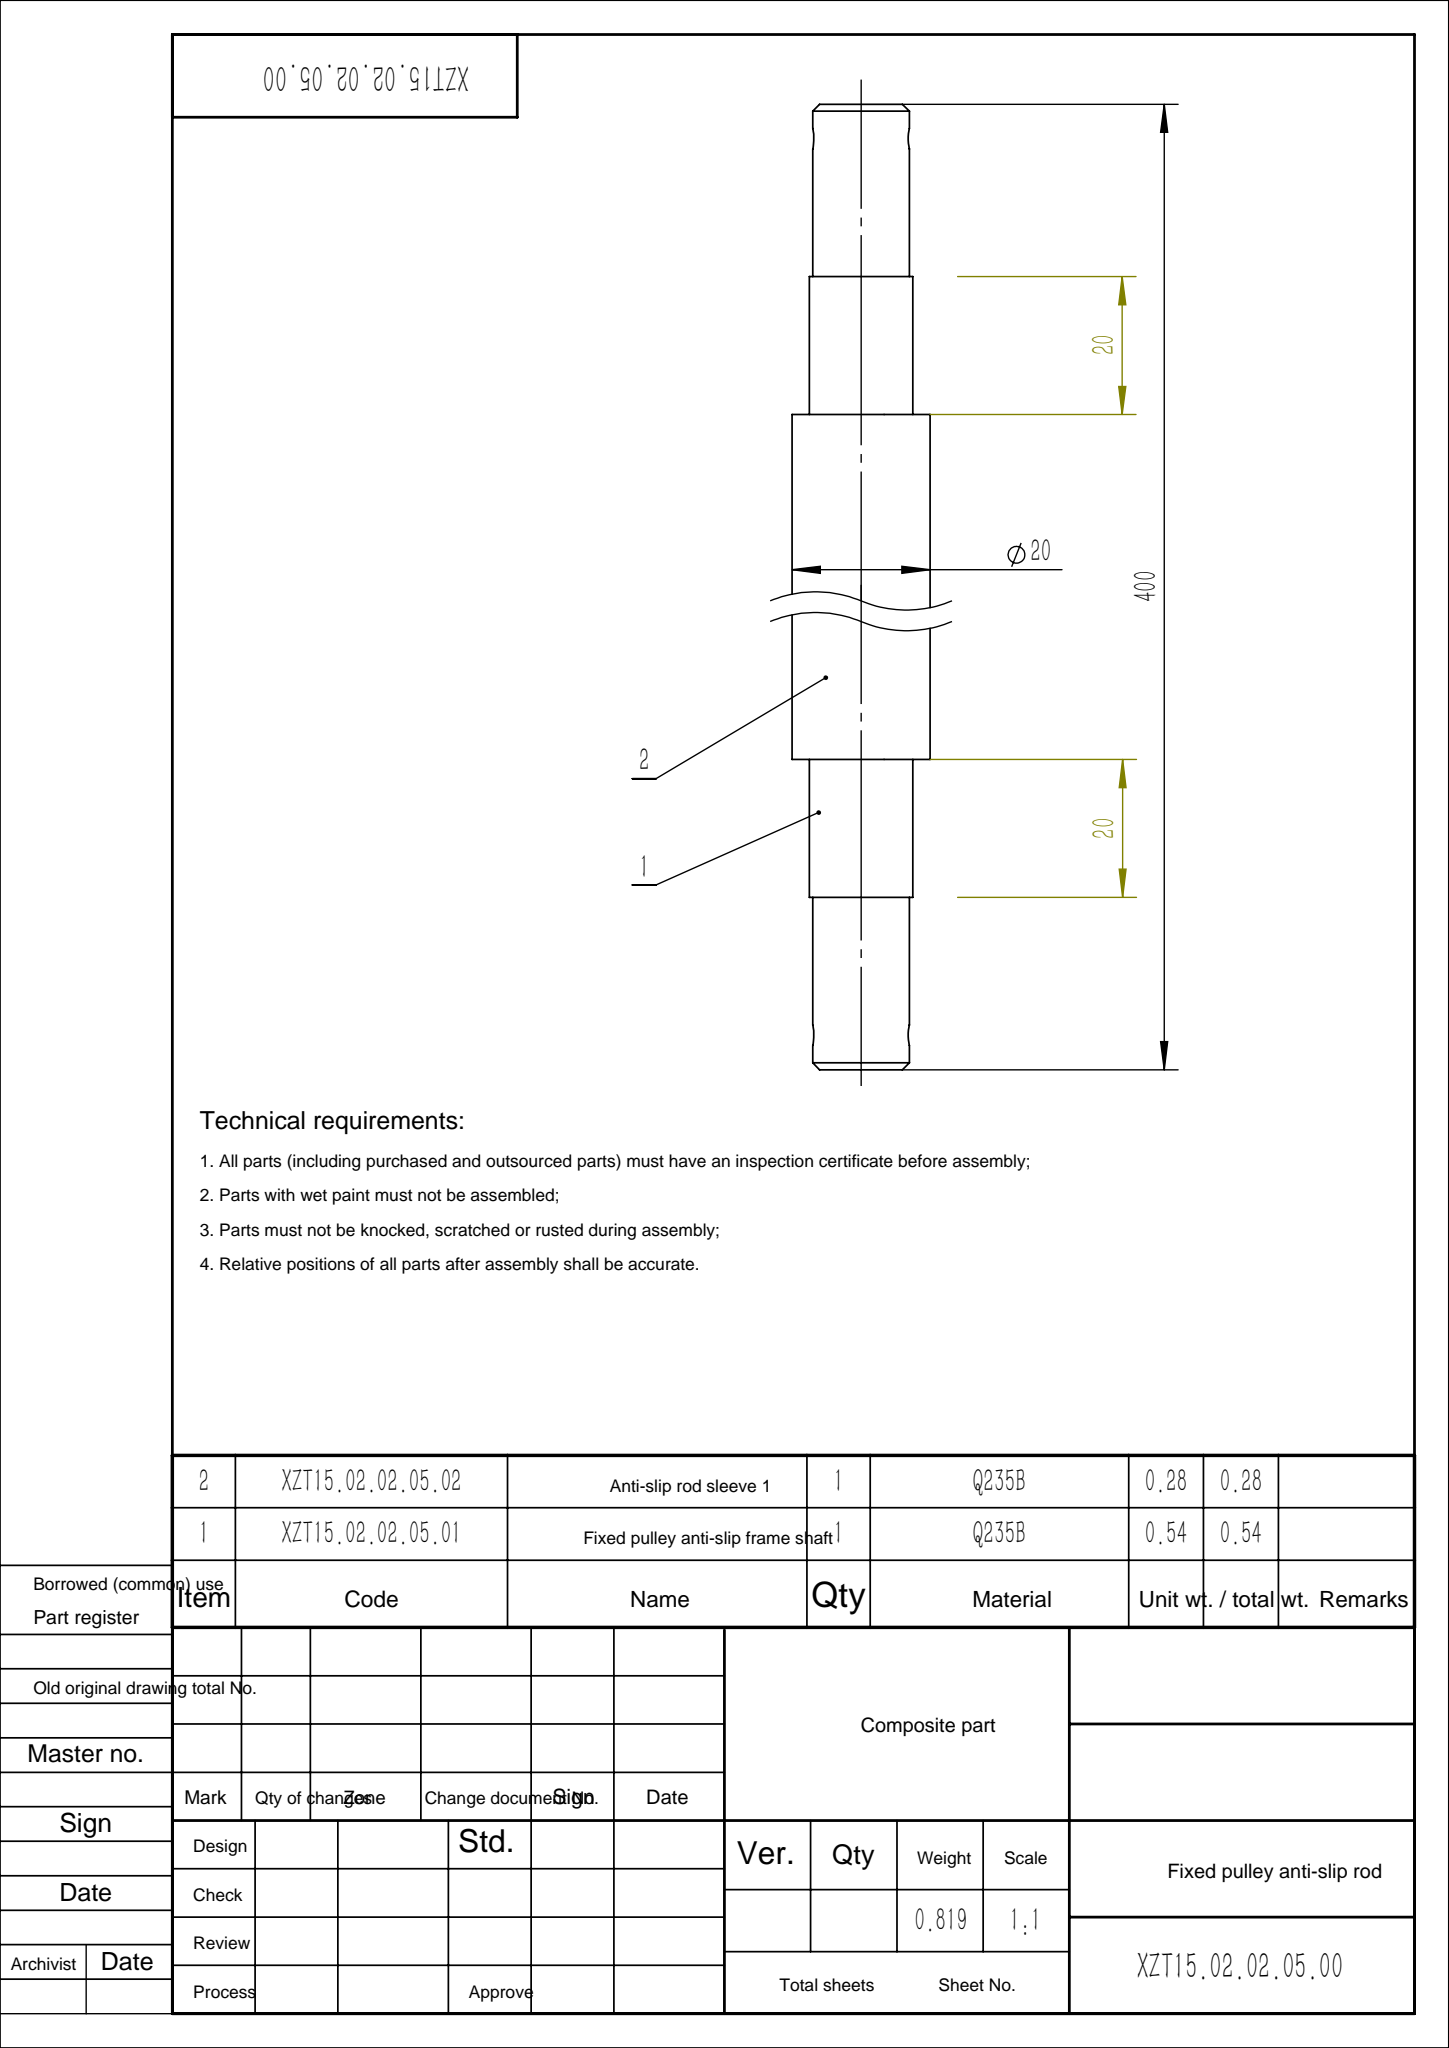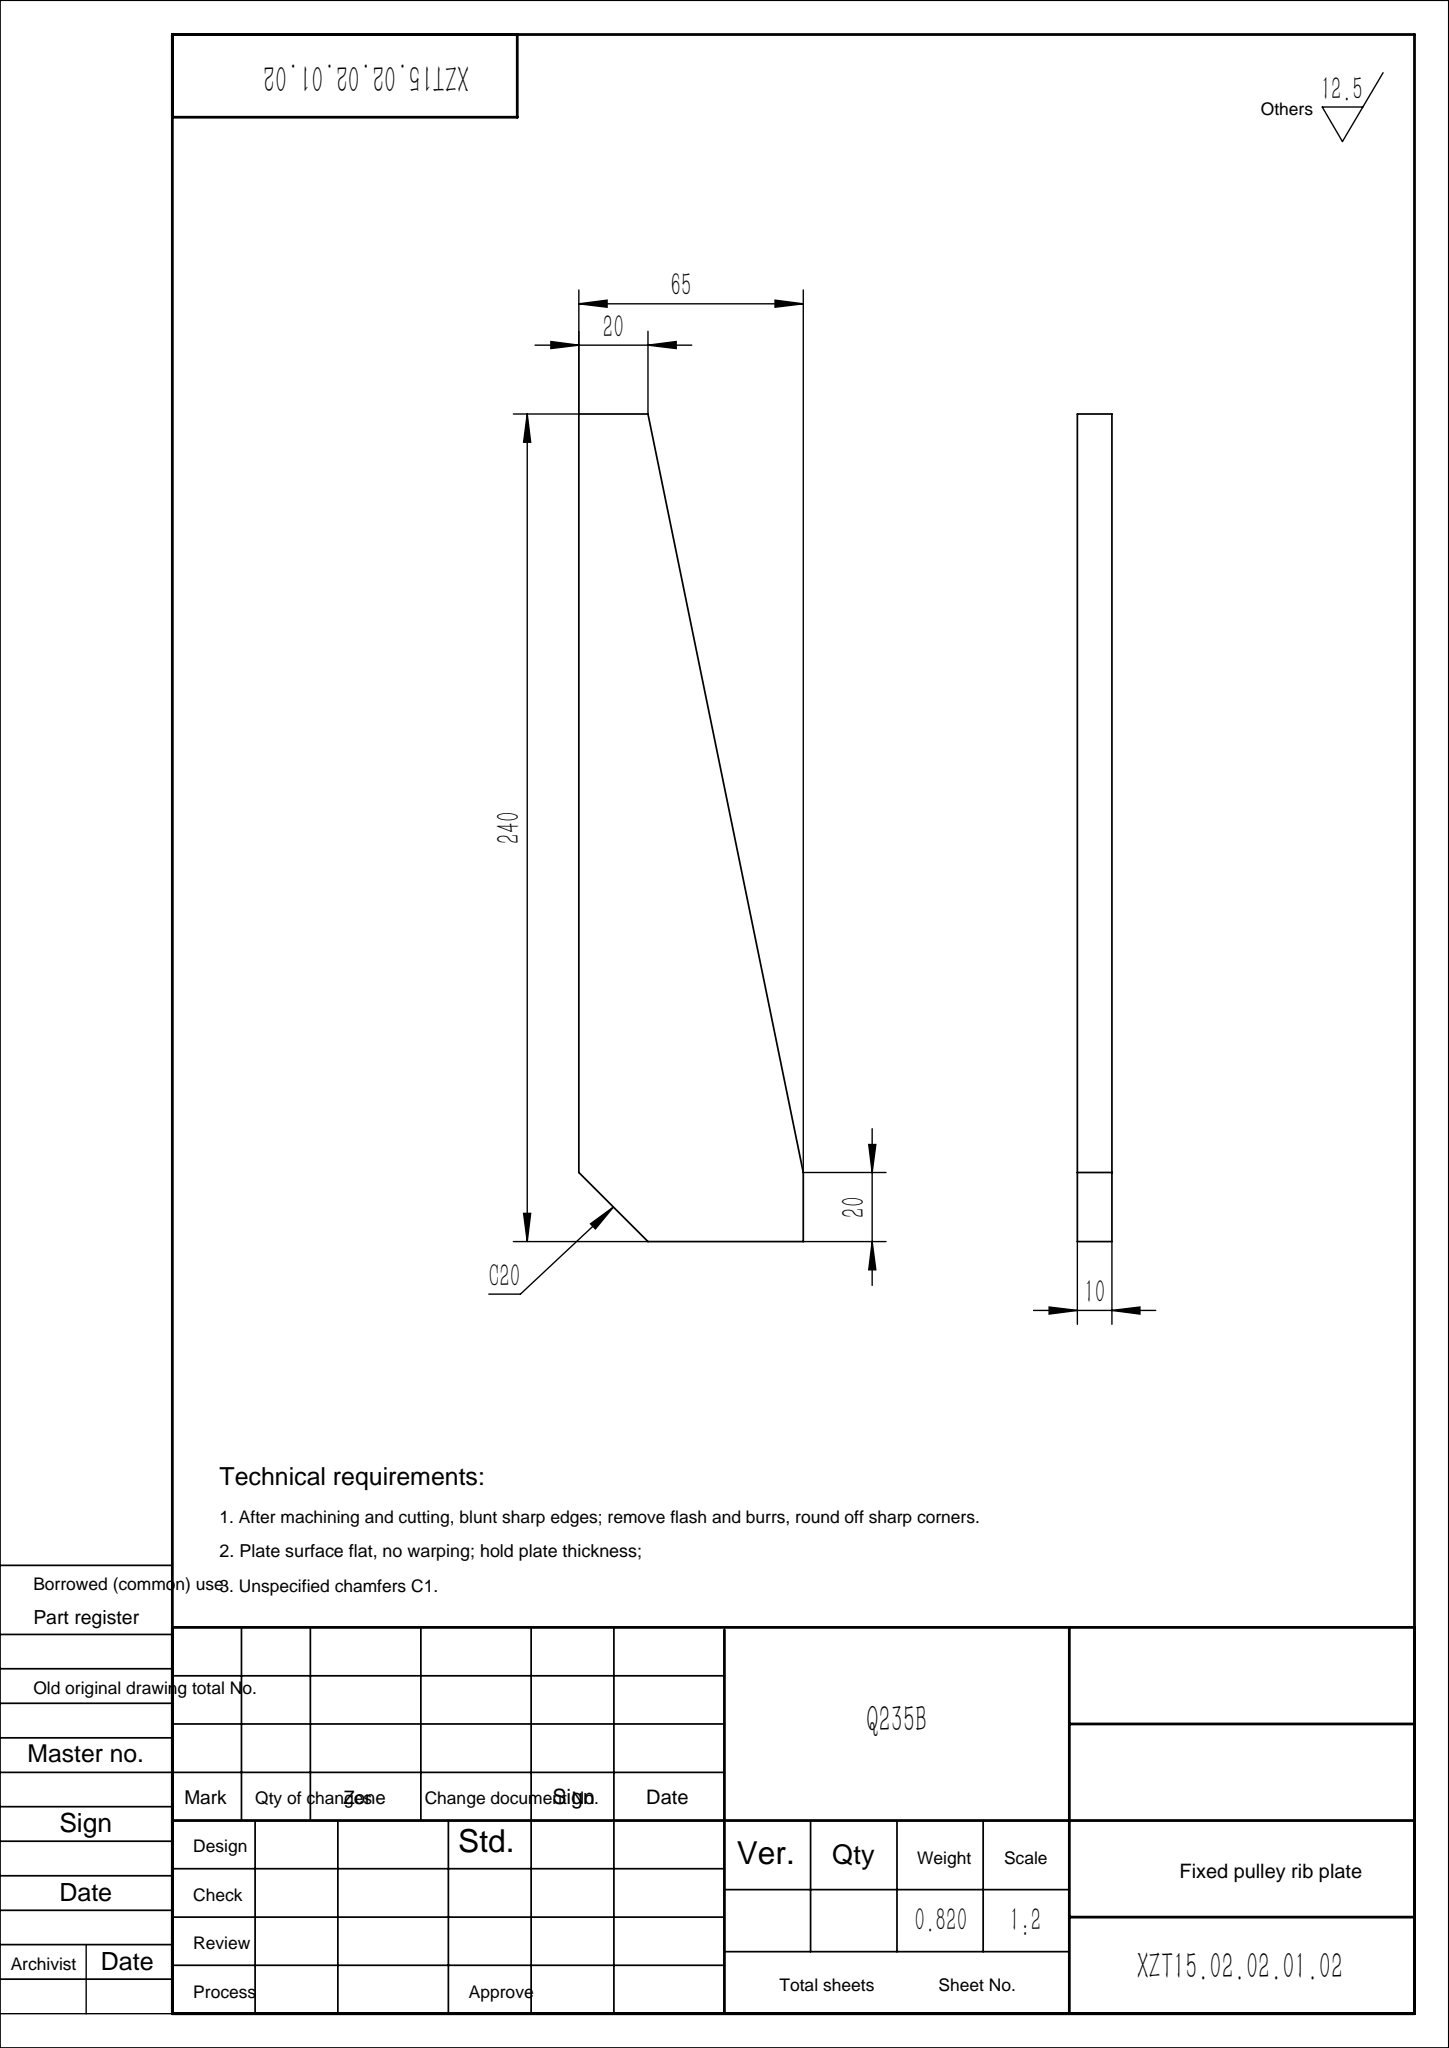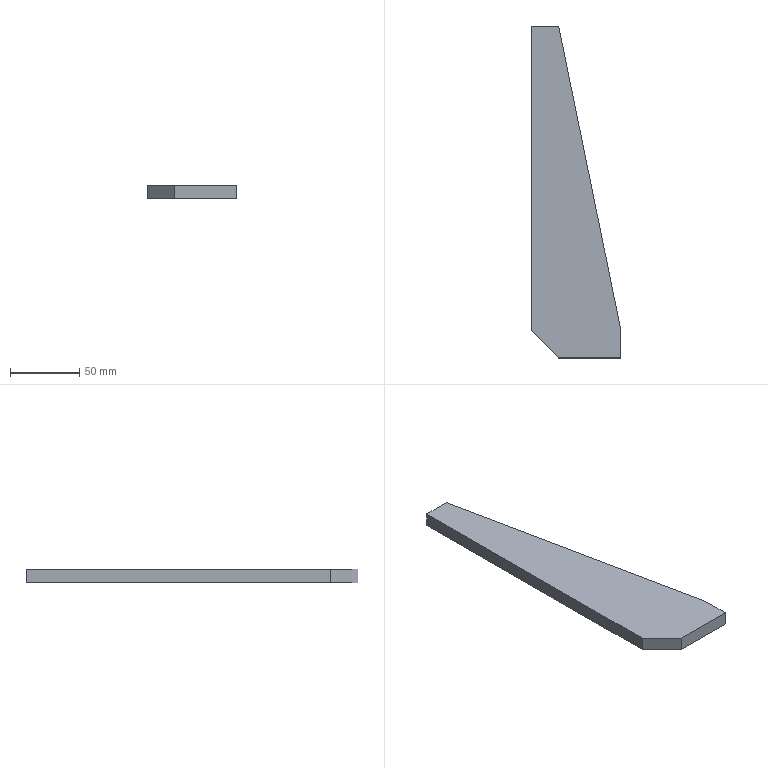Part | SolidWorks | features Chamfer 1, Extrusion 1 | 1 solid | 8 faces | box 65 x 240 x 10 mm | volume 104500 mm3 | plane 8
STEP:
#1=CARTESIAN_POINT('',(0.,240.,-5.));
#2=VERTEX_POINT('',#1);
#3=CARTESIAN_POINT('',(0.,20.,-5.));
#4=VERTEX_POINT('',#3);
#5=CARTESIAN_POINT('',(0.,240.,-5.));
#6=DIRECTION('',(0.,-1.,0.));
#7=VECTOR('',#6,1000.);
#8=LINE('',#5,#7);
#9=EDGE_CURVE('',#2,#4,#8,.T.);
#10=ORIENTED_EDGE('',*,*,#9,.T.);
#11=CARTESIAN_POINT('',(0.,20.,5.));
#12=VERTEX_POINT('',#11);
#13=CARTESIAN_POINT('',(0.,20.,5.));
#14=DIRECTION('',(0.,0.,1.));
#15=VECTOR('',#14,1000.);
#16=LINE('',#13,#15);
#17=EDGE_CURVE('',#4,#12,#16,.T.);
#18=ORIENTED_EDGE('',*,*,#17,.T.);
#19=CARTESIAN_POINT('',(0.,240.,5.));
#20=VERTEX_POINT('',#19);
#21=CARTESIAN_POINT('',(0.,240.,5.));
#22=DIRECTION('',(0.,-1.,0.));
#23=VECTOR('',#22,1000.);
#24=LINE('',#21,#23);
#25=EDGE_CURVE('',#20,#12,#24,.T.);
#26=ORIENTED_EDGE('',*,*,#25,.F.);
#27=CARTESIAN_POINT('',(0.,240.,5.));
#28=DIRECTION('',(0.,0.,-1.));
#29=VECTOR('',#28,1000.);
#30=LINE('',#27,#29);
#31=EDGE_CURVE('',#20,#2,#30,.T.);
#32=ORIENTED_EDGE('',*,*,#31,.T.);
#33=EDGE_LOOP('',(#10,#18,#26,#32));
#34=FACE_OUTER_BOUND('',#33,.T.);
#35=CARTESIAN_POINT('',(0.,240.,5.));
#36=DIRECTION('',(1.,0.,0.));
#37=DIRECTION('',(0.,1.,0.));
#38=AXIS2_PLACEMENT_3D('',#35,#36,#37);
#39=PLANE('',#38);
#40=ADVANCED_FACE('',(#34),#39,.F.);
#41=CARTESIAN_POINT('',(20.,0.,5.));
#42=VERTEX_POINT('',#41);
#43=CARTESIAN_POINT('',(65.,0.,5.));
#44=VERTEX_POINT('',#43);
#45=CARTESIAN_POINT('',(0.,0.,5.));
#46=DIRECTION('',(1.,0.,0.));
#47=VECTOR('',#46,1000.);
#48=LINE('',#45,#47);
#49=EDGE_CURVE('',#42,#44,#48,.T.);
#50=ORIENTED_EDGE('',*,*,#49,.F.);
#51=CARTESIAN_POINT('',(20.,0.,-5.));
#52=VERTEX_POINT('',#51);
#53=CARTESIAN_POINT('',(20.,0.,5.));
#54=DIRECTION('',(0.,0.,-1.));
#55=VECTOR('',#54,1000.);
#56=LINE('',#53,#55);
#57=EDGE_CURVE('',#42,#52,#56,.T.);
#58=ORIENTED_EDGE('',*,*,#57,.T.);
#59=CARTESIAN_POINT('',(65.,0.,-5.));
#60=VERTEX_POINT('',#59);
#61=CARTESIAN_POINT('',(0.,0.,-5.));
#62=DIRECTION('',(1.,0.,0.));
#63=VECTOR('',#62,1000.);
#64=LINE('',#61,#63);
#65=EDGE_CURVE('',#52,#60,#64,.T.);
#66=ORIENTED_EDGE('',*,*,#65,.T.);
#67=CARTESIAN_POINT('',(65.,0.,5.));
#68=DIRECTION('',(0.,0.,-1.));
#69=VECTOR('',#68,1000.);
#70=LINE('',#67,#69);
#71=EDGE_CURVE('',#44,#60,#70,.T.);
#72=ORIENTED_EDGE('',*,*,#71,.F.);
#73=EDGE_LOOP('',(#50,#58,#66,#72));
#74=FACE_OUTER_BOUND('',#73,.T.);
#75=CARTESIAN_POINT('',(0.,0.,5.));
#76=DIRECTION('',(0.,1.,0.));
#77=DIRECTION('',(0.,0.,1.));
#78=AXIS2_PLACEMENT_3D('',#75,#76,#77);
#79=PLANE('',#78);
#80=ADVANCED_FACE('',(#74),#79,.F.);
#81=CARTESIAN_POINT('',(65.,20.,-5.));
#82=VERTEX_POINT('',#81);
#83=CARTESIAN_POINT('',(65.,0.,-5.));
#84=DIRECTION('',(0.,1.,0.));
#85=VECTOR('',#84,1000.);
#86=LINE('',#83,#85);
#87=EDGE_CURVE('',#60,#82,#86,.T.);
#88=ORIENTED_EDGE('',*,*,#87,.T.);
#89=CARTESIAN_POINT('',(65.,20.,5.));
#90=VERTEX_POINT('',#89);
#91=CARTESIAN_POINT('',(65.,20.,5.));
#92=DIRECTION('',(0.,0.,-1.));
#93=VECTOR('',#92,1000.);
#94=LINE('',#91,#93);
#95=EDGE_CURVE('',#90,#82,#94,.T.);
#96=ORIENTED_EDGE('',*,*,#95,.F.);
#97=CARTESIAN_POINT('',(65.,0.,5.));
#98=DIRECTION('',(0.,1.,0.));
#99=VECTOR('',#98,1000.);
#100=LINE('',#97,#99);
#101=EDGE_CURVE('',#44,#90,#100,.T.);
#102=ORIENTED_EDGE('',*,*,#101,.F.);
#103=ORIENTED_EDGE('',*,*,#71,.T.);
#104=EDGE_LOOP('',(#88,#96,#102,#103));
#105=FACE_OUTER_BOUND('',#104,.T.);
#106=CARTESIAN_POINT('',(65.,0.,5.));
#107=DIRECTION('',(-1.,0.,0.));
#108=DIRECTION('',(0.,0.,1.));
#109=AXIS2_PLACEMENT_3D('',#106,#107,#108);
#110=PLANE('',#109);
#111=ADVANCED_FACE('',(#105),#110,.F.);
#112=CARTESIAN_POINT('',(20.,240.,-5.));
#113=VERTEX_POINT('',#112);
#114=CARTESIAN_POINT('',(65.,20.,-5.));
#115=DIRECTION('',(-0.2004,0.9797,0.));
#116=VECTOR('',#115,1000.);
#117=LINE('',#114,#116);
#118=EDGE_CURVE('',#82,#113,#117,.T.);
#119=ORIENTED_EDGE('',*,*,#118,.T.);
#120=CARTESIAN_POINT('',(20.,240.,5.));
#121=VERTEX_POINT('',#120);
#122=CARTESIAN_POINT('',(20.,240.,5.));
#123=DIRECTION('',(0.,0.,-1.));
#124=VECTOR('',#123,1000.);
#125=LINE('',#122,#124);
#126=EDGE_CURVE('',#121,#113,#125,.T.);
#127=ORIENTED_EDGE('',*,*,#126,.F.);
#128=CARTESIAN_POINT('',(65.,20.,5.));
#129=DIRECTION('',(-0.2004,0.9797,0.));
#130=VECTOR('',#129,1000.);
#131=LINE('',#128,#130);
#132=EDGE_CURVE('',#90,#121,#131,.T.);
#133=ORIENTED_EDGE('',*,*,#132,.F.);
#134=ORIENTED_EDGE('',*,*,#95,.T.);
#135=EDGE_LOOP('',(#119,#127,#133,#134));
#136=FACE_OUTER_BOUND('',#135,.T.);
#137=CARTESIAN_POINT('',(65.,20.,5.));
#138=DIRECTION('',(-0.9797,-0.2004,0.));
#139=DIRECTION('',(0.2004,-0.9797,0.));
#140=AXIS2_PLACEMENT_3D('',#137,#138,#139);
#141=PLANE('',#140);
#142=ADVANCED_FACE('',(#136),#141,.F.);
#143=CARTESIAN_POINT('',(20.,240.,-5.));
#144=DIRECTION('',(-1.,0.,0.));
#145=VECTOR('',#144,1000.);
#146=LINE('',#143,#145);
#147=EDGE_CURVE('',#113,#2,#146,.T.);
#148=ORIENTED_EDGE('',*,*,#147,.T.);
#149=ORIENTED_EDGE('',*,*,#31,.F.);
#150=CARTESIAN_POINT('',(20.,240.,5.));
#151=DIRECTION('',(-1.,0.,0.));
#152=VECTOR('',#151,1000.);
#153=LINE('',#150,#152);
#154=EDGE_CURVE('',#121,#20,#153,.T.);
#155=ORIENTED_EDGE('',*,*,#154,.F.);
#156=ORIENTED_EDGE('',*,*,#126,.T.);
#157=EDGE_LOOP('',(#148,#149,#155,#156));
#158=FACE_OUTER_BOUND('',#157,.T.);
#159=CARTESIAN_POINT('',(20.,240.,5.));
#160=DIRECTION('',(0.,-1.,0.));
#161=DIRECTION('',(0.,0.,-1.));
#162=AXIS2_PLACEMENT_3D('',#159,#160,#161);
#163=PLANE('',#162);
#164=ADVANCED_FACE('',(#158),#163,.F.);
#165=ORIENTED_EDGE('',*,*,#25,.T.);
#166=CARTESIAN_POINT('',(10.,10.,5.));
#167=DIRECTION('',(0.7071,-0.7071,0.));
#168=VECTOR('',#167,1000.);
#169=LINE('',#166,#168);
#170=EDGE_CURVE('',#12,#42,#169,.T.);
#171=ORIENTED_EDGE('',*,*,#170,.T.);
#172=ORIENTED_EDGE('',*,*,#49,.T.);
#173=ORIENTED_EDGE('',*,*,#101,.T.);
#174=ORIENTED_EDGE('',*,*,#132,.T.);
#175=ORIENTED_EDGE('',*,*,#154,.T.);
#176=EDGE_LOOP('',(#165,#171,#172,#173,#174,#175));
#177=FACE_OUTER_BOUND('',#176,.T.);
#178=CARTESIAN_POINT('',(0.,0.,5.));
#179=DIRECTION('',(0.,0.,1.));
#180=DIRECTION('',(1.,0.,0.));
#181=AXIS2_PLACEMENT_3D('',#178,#179,#180);
#182=PLANE('',#181);
#183=ADVANCED_FACE('',(#177),#182,.T.);
#184=ORIENTED_EDGE('',*,*,#65,.F.);
#185=CARTESIAN_POINT('',(20.,0.,-5.));
#186=DIRECTION('',(-0.7071,0.7071,0.));
#187=VECTOR('',#186,1000.);
#188=LINE('',#185,#187);
#189=EDGE_CURVE('',#52,#4,#188,.T.);
#190=ORIENTED_EDGE('',*,*,#189,.T.);
#191=ORIENTED_EDGE('',*,*,#9,.F.);
#192=ORIENTED_EDGE('',*,*,#147,.F.);
#193=ORIENTED_EDGE('',*,*,#118,.F.);
#194=ORIENTED_EDGE('',*,*,#87,.F.);
#195=EDGE_LOOP('',(#184,#190,#191,#192,#193,#194));
#196=FACE_OUTER_BOUND('',#195,.T.);
#197=CARTESIAN_POINT('',(0.,0.,-5.));
#198=DIRECTION('',(0.,0.,1.));
#199=DIRECTION('',(1.,0.,0.));
#200=AXIS2_PLACEMENT_3D('',#197,#198,#199);
#201=PLANE('',#200);
#202=ADVANCED_FACE('',(#196),#201,.F.);
#203=ORIENTED_EDGE('',*,*,#170,.F.);
#204=ORIENTED_EDGE('',*,*,#17,.F.);
#205=ORIENTED_EDGE('',*,*,#189,.F.);
#206=ORIENTED_EDGE('',*,*,#57,.F.);
#207=EDGE_LOOP('',(#203,#204,#205,#206));
#208=FACE_OUTER_BOUND('',#207,.T.);
#209=CARTESIAN_POINT('',(20.,0.,5.));
#210=DIRECTION('',(0.7071,0.7071,0.));
#211=DIRECTION('',(0.,0.,-1.));
#212=AXIS2_PLACEMENT_3D('',#209,#210,#211);
#213=PLANE('',#212);
#214=ADVANCED_FACE('',(#208),#213,.F.);
#215=CLOSED_SHELL('',(#40,#80,#111,#142,#164,#183,#202,#214));
#216=MANIFOLD_SOLID_BREP('',#215);
#217=CARTESIAN_POINT('',(0.,0.,0.));
#218=DIRECTION('',(0.,0.,1.));
#219=DIRECTION('',(1.,0.,0.));
#220=AXIS2_PLACEMENT_3D('',#217,#218,#219);
#221=(LENGTH_UNIT()NAMED_UNIT(*)SI_UNIT(.MILLI.,.METRE.));
#222=UNCERTAINTY_MEASURE_WITH_UNIT(LENGTH_MEASURE(0.00001),#221,'','');
#223=(NAMED_UNIT(*)PLANE_ANGLE_UNIT()SI_UNIT($,.RADIAN.));
#224=(NAMED_UNIT(*)SI_UNIT($,.STERADIAN.)SOLID_ANGLE_UNIT());
#225=(GEOMETRIC_REPRESENTATION_CONTEXT(3)GLOBAL_UNCERTAINTY_ASSIGNED_CONTEXT((#222))GLOBAL_UNIT_ASSIGNED_CONTEXT((#221,#223,#224))REPRESENTATION_CONTEXT('',''));
#226=ADVANCED_BREP_SHAPE_REPRESENTATION('',(#216,#220),#225);